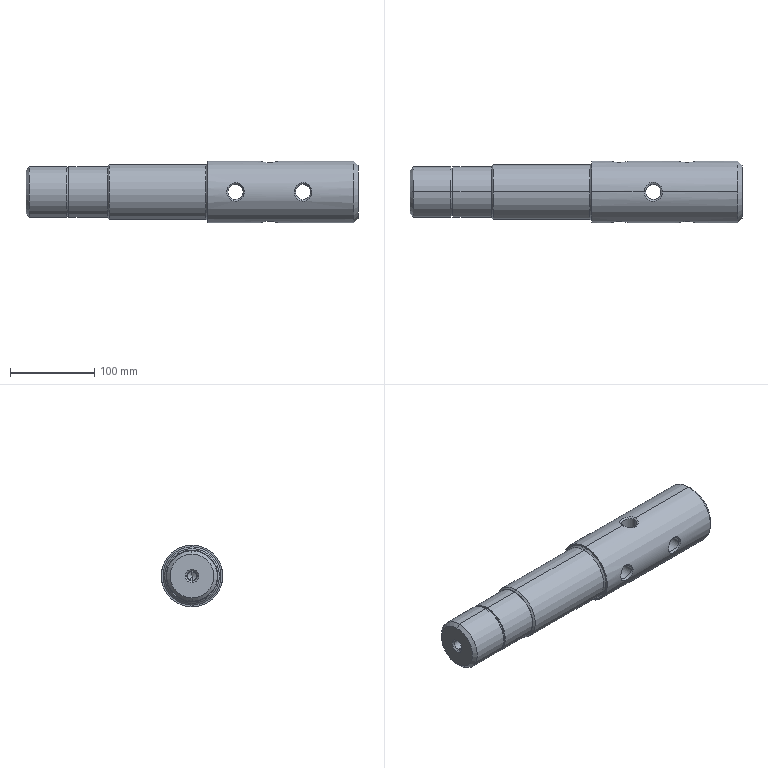Part | STEP file | Input 25 | 1 solid | 51 faces | box 393 x 73 x 73 mm | volume 1345676 mm3 | cylinder 20 | spline 12 | cone 12 | plane 7 | commonest cylinder face diameters 18 x6 60 x4 10.2 x2 12 x2 57 x2 65 x2